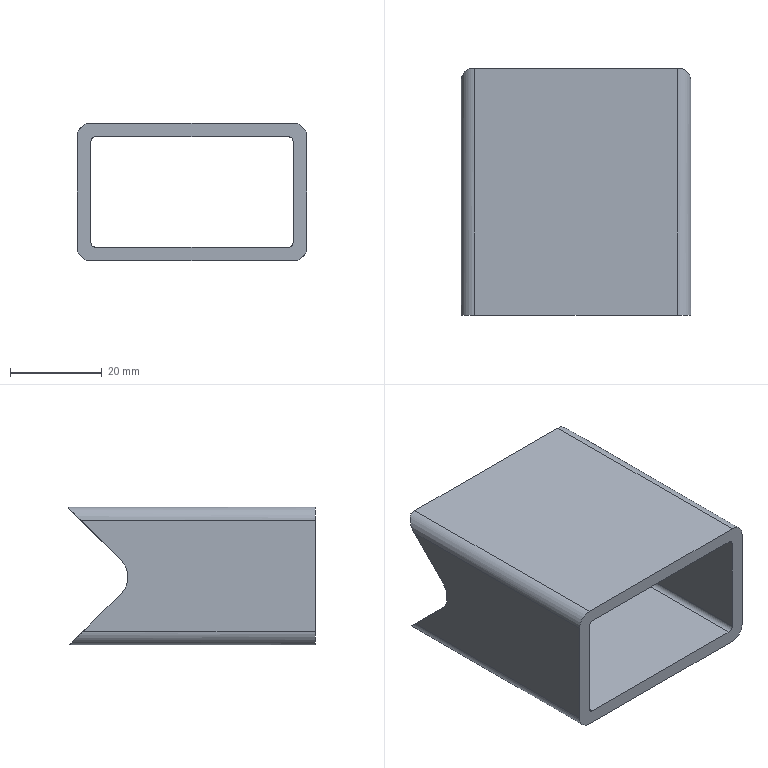Part | SolidWorks | features Fillet 2, Extrusion 1, ICE 1, Shell 1 | 1 solid | 22 faces | box 50 x 53.7 x 30 mm | volume 21768 mm3 | plane 12 | cylinder 10 | commonest cylinder face diameters 2 x4 6 x4 10 x2
STEP:
#1=CARTESIAN_POINT('',(23.24,26.85,29.732));
#2=VERTEX_POINT('',#1);
#3=CARTESIAN_POINT('',(-23.24,26.85,29.732));
#4=VERTEX_POINT('',#3);
#5=CARTESIAN_POINT('',(-25.,26.85,29.732));
#6=DIRECTION('',(-1.,0.,0.));
#7=VECTOR('',#6,1000.);
#8=LINE('',#5,#7);
#9=EDGE_CURVE('',#2,#4,#8,.T.);
#10=ORIENTED_EDGE('',*,*,#9,.T.);
#11=CARTESIAN_POINT('',(-22.,26.85,30.));
#12=VERTEX_POINT('',#11);
#13=CARTESIAN_POINT('',(-22.,26.85,27.));
#14=DIRECTION('',(0.,1.,0.));
#15=DIRECTION('',(0.,0.,-1.));
#16=AXIS2_PLACEMENT_3D('',#13,#14,#15);
#17=CIRCLE('',#16,3.);
#18=EDGE_CURVE('',#4,#12,#17,.T.);
#19=ORIENTED_EDGE('',*,*,#18,.T.);
#20=CARTESIAN_POINT('',(22.,26.85,30.));
#21=VERTEX_POINT('',#20);
#22=CARTESIAN_POINT('',(-25.,26.85,30.));
#23=DIRECTION('',(-1.,0.,0.));
#24=VECTOR('',#23,1000.);
#25=LINE('',#22,#24);
#26=EDGE_CURVE('',#21,#12,#25,.T.);
#27=ORIENTED_EDGE('',*,*,#26,.F.);
#28=CARTESIAN_POINT('',(22.,26.85,27.));
#29=DIRECTION('',(0.,1.,0.));
#30=DIRECTION('',(0.,0.,-1.));
#31=AXIS2_PLACEMENT_3D('',#28,#29,#30);
#32=CIRCLE('',#31,3.);
#33=EDGE_CURVE('',#21,#2,#32,.T.);
#34=ORIENTED_EDGE('',*,*,#33,.T.);
#35=EDGE_LOOP('',(#10,#19,#27,#34));
#36=FACE_OUTER_BOUND('',#35,.T.);
#37=CARTESIAN_POINT('',(-25.,26.85,30.));
#38=DIRECTION('',(0.,-1.,0.));
#39=DIRECTION('',(0.,0.,-1.));
#40=AXIS2_PLACEMENT_3D('',#37,#38,#39);
#41=PLANE('',#40);
#42=ADVANCED_FACE('',(#36),#41,.F.);
#43=CARTESIAN_POINT('',(-25.,-26.85,27.));
#44=VERTEX_POINT('',#43);
#45=CARTESIAN_POINT('',(-25.,-26.85,3.));
#46=VERTEX_POINT('',#45);
#47=CARTESIAN_POINT('',(-25.,-26.85,30.));
#48=DIRECTION('',(0.,0.,-1.));
#49=VECTOR('',#48,1000.);
#50=LINE('',#47,#49);
#51=EDGE_CURVE('',#44,#46,#50,.T.);
#52=ORIENTED_EDGE('',*,*,#51,.T.);
#53=CARTESIAN_POINT('',(-22.,-26.85,0.));
#54=VERTEX_POINT('',#53);
#55=CARTESIAN_POINT('',(-22.,-26.85,3.));
#56=DIRECTION('',(0.,-1.,0.));
#57=DIRECTION('',(0.,0.,1.));
#58=AXIS2_PLACEMENT_3D('',#55,#56,#57);
#59=CIRCLE('',#58,3.);
#60=EDGE_CURVE('',#46,#54,#59,.T.);
#61=ORIENTED_EDGE('',*,*,#60,.T.);
#62=CARTESIAN_POINT('',(22.,-26.85,0.));
#63=VERTEX_POINT('',#62);
#64=CARTESIAN_POINT('',(-25.,-26.85,0.));
#65=DIRECTION('',(1.,0.,0.));
#66=VECTOR('',#65,1000.);
#67=LINE('',#64,#66);
#68=EDGE_CURVE('',#54,#63,#67,.T.);
#69=ORIENTED_EDGE('',*,*,#68,.T.);
#70=CARTESIAN_POINT('',(25.,-26.85,3.));
#71=VERTEX_POINT('',#70);
#72=CARTESIAN_POINT('',(22.,-26.85,3.));
#73=DIRECTION('',(0.,-1.,0.));
#74=DIRECTION('',(0.,0.,1.));
#75=AXIS2_PLACEMENT_3D('',#72,#73,#74);
#76=CIRCLE('',#75,3.);
#77=EDGE_CURVE('',#63,#71,#76,.T.);
#78=ORIENTED_EDGE('',*,*,#77,.T.);
#79=CARTESIAN_POINT('',(25.,-26.85,27.));
#80=VERTEX_POINT('',#79);
#81=CARTESIAN_POINT('',(25.,-26.85,30.));
#82=DIRECTION('',(0.,0.,-1.));
#83=VECTOR('',#82,1000.);
#84=LINE('',#81,#83);
#85=EDGE_CURVE('',#80,#71,#84,.T.);
#86=ORIENTED_EDGE('',*,*,#85,.F.);
#87=CARTESIAN_POINT('',(22.,-26.85,30.));
#88=VERTEX_POINT('',#87);
#89=CARTESIAN_POINT('',(22.,-26.85,27.));
#90=DIRECTION('',(0.,-1.,0.));
#91=DIRECTION('',(0.,0.,1.));
#92=AXIS2_PLACEMENT_3D('',#89,#90,#91);
#93=CIRCLE('',#92,3.);
#94=EDGE_CURVE('',#80,#88,#93,.T.);
#95=ORIENTED_EDGE('',*,*,#94,.T.);
#96=CARTESIAN_POINT('',(-22.,-26.85,30.));
#97=VERTEX_POINT('',#96);
#98=CARTESIAN_POINT('',(-25.,-26.85,30.));
#99=DIRECTION('',(1.,0.,0.));
#100=VECTOR('',#99,1000.);
#101=LINE('',#98,#100);
#102=EDGE_CURVE('',#97,#88,#101,.T.);
#103=ORIENTED_EDGE('',*,*,#102,.F.);
#104=CARTESIAN_POINT('',(-22.,-26.85,27.));
#105=DIRECTION('',(0.,-1.,0.));
#106=DIRECTION('',(0.,0.,1.));
#107=AXIS2_PLACEMENT_3D('',#104,#105,#106);
#108=CIRCLE('',#107,3.);
#109=EDGE_CURVE('',#97,#44,#108,.T.);
#110=ORIENTED_EDGE('',*,*,#109,.T.);
#111=EDGE_LOOP('',(#52,#61,#69,#78,#86,#95,#103,#110));
#112=FACE_OUTER_BOUND('',#111,.T.);
#113=CARTESIAN_POINT('',(-21.,-26.85,3.));
#114=VERTEX_POINT('',#113);
#115=CARTESIAN_POINT('',(21.,-26.85,3.));
#116=VERTEX_POINT('',#115);
#117=CARTESIAN_POINT('',(-25.,-26.85,3.));
#118=DIRECTION('',(1.,0.,0.));
#119=VECTOR('',#118,1000.);
#120=LINE('',#117,#119);
#121=EDGE_CURVE('',#114,#116,#120,.T.);
#122=ORIENTED_EDGE('',*,*,#121,.F.);
#123=CARTESIAN_POINT('',(-22.,-26.85,4.));
#124=VERTEX_POINT('',#123);
#125=CARTESIAN_POINT('',(-21.,-26.85,4.));
#126=DIRECTION('',(0.,1.,0.));
#127=DIRECTION('',(0.,0.,1.));
#128=AXIS2_PLACEMENT_3D('',#125,#126,#127);
#129=CIRCLE('',#128,1.);
#130=EDGE_CURVE('',#114,#124,#129,.T.);
#131=ORIENTED_EDGE('',*,*,#130,.T.);
#132=CARTESIAN_POINT('',(-22.,-26.85,26.));
#133=VERTEX_POINT('',#132);
#134=CARTESIAN_POINT('',(-22.,-26.85,30.));
#135=DIRECTION('',(0.,0.,-1.));
#136=VECTOR('',#135,1000.);
#137=LINE('',#134,#136);
#138=EDGE_CURVE('',#133,#124,#137,.T.);
#139=ORIENTED_EDGE('',*,*,#138,.F.);
#140=CARTESIAN_POINT('',(-21.,-26.85,27.));
#141=VERTEX_POINT('',#140);
#142=CARTESIAN_POINT('',(-21.,-26.85,26.));
#143=DIRECTION('',(0.,1.,0.));
#144=DIRECTION('',(0.,0.,1.));
#145=AXIS2_PLACEMENT_3D('',#142,#143,#144);
#146=CIRCLE('',#145,1.);
#147=EDGE_CURVE('',#133,#141,#146,.T.);
#148=ORIENTED_EDGE('',*,*,#147,.T.);
#149=CARTESIAN_POINT('',(21.,-26.85,27.));
#150=VERTEX_POINT('',#149);
#151=CARTESIAN_POINT('',(-25.,-26.85,27.));
#152=DIRECTION('',(1.,0.,0.));
#153=VECTOR('',#152,1000.);
#154=LINE('',#151,#153);
#155=EDGE_CURVE('',#141,#150,#154,.T.);
#156=ORIENTED_EDGE('',*,*,#155,.T.);
#157=CARTESIAN_POINT('',(22.,-26.85,26.));
#158=VERTEX_POINT('',#157);
#159=CARTESIAN_POINT('',(21.,-26.85,26.));
#160=DIRECTION('',(0.,1.,0.));
#161=DIRECTION('',(0.,0.,1.));
#162=AXIS2_PLACEMENT_3D('',#159,#160,#161);
#163=CIRCLE('',#162,1.);
#164=EDGE_CURVE('',#150,#158,#163,.T.);
#165=ORIENTED_EDGE('',*,*,#164,.T.);
#166=CARTESIAN_POINT('',(22.,-26.85,4.));
#167=VERTEX_POINT('',#166);
#168=CARTESIAN_POINT('',(22.,-26.85,30.));
#169=DIRECTION('',(0.,0.,-1.));
#170=VECTOR('',#169,1000.);
#171=LINE('',#168,#170);
#172=EDGE_CURVE('',#158,#167,#171,.T.);
#173=ORIENTED_EDGE('',*,*,#172,.T.);
#174=CARTESIAN_POINT('',(21.,-26.85,4.));
#175=DIRECTION('',(0.,1.,0.));
#176=DIRECTION('',(0.,0.,1.));
#177=AXIS2_PLACEMENT_3D('',#174,#175,#176);
#178=CIRCLE('',#177,1.);
#179=EDGE_CURVE('',#167,#116,#178,.T.);
#180=ORIENTED_EDGE('',*,*,#179,.T.);
#181=EDGE_LOOP('',(#122,#131,#139,#148,#156,#165,#173,#180));
#182=FACE_BOUND('',#181,.T.);
#183=CARTESIAN_POINT('',(-25.,-26.85,30.));
#184=DIRECTION('',(0.,1.,0.));
#185=DIRECTION('',(0.,0.,1.));
#186=AXIS2_PLACEMENT_3D('',#183,#184,#185);
#187=PLANE('',#186);
#188=ADVANCED_FACE('',(#112,#182),#187,.F.);
#189=ORIENTED_EDGE('',*,*,#85,.T.);
#190=CARTESIAN_POINT('',(25.,23.613,3.));
#191=VERTEX_POINT('',#190);
#192=CARTESIAN_POINT('',(25.,26.85,3.));
#193=DIRECTION('',(0.,1.,0.));
#194=VECTOR('',#193,1000.);
#195=LINE('',#192,#194);
#196=EDGE_CURVE('',#71,#191,#195,.T.);
#197=ORIENTED_EDGE('',*,*,#196,.T.);
#198=CARTESIAN_POINT('',(25.,15.401,11.212));
#199=VERTEX_POINT('',#198);
#200=CARTESIAN_POINT('',(25.,15.401,11.212));
#201=DIRECTION('',(0.,0.7071,-0.7071));
#202=VECTOR('',#201,1000.);
#203=LINE('',#200,#202);
#204=EDGE_CURVE('',#199,#191,#203,.T.);
#205=ORIENTED_EDGE('',*,*,#204,.F.);
#206=CARTESIAN_POINT('',(25.,15.401,18.283));
#207=VERTEX_POINT('',#206);
#208=CARTESIAN_POINT('',(25.,18.937,14.748));
#209=DIRECTION('',(1.,0.,0.));
#210=DIRECTION('',(0.,1.,0.));
#211=AXIS2_PLACEMENT_3D('',#208,#209,#210);
#212=CIRCLE('',#211,5.);
#213=EDGE_CURVE('',#207,#199,#212,.T.);
#214=ORIENTED_EDGE('',*,*,#213,.F.);
#215=CARTESIAN_POINT('',(25.,24.118,27.));
#216=VERTEX_POINT('',#215);
#217=CARTESIAN_POINT('',(25.,15.401,18.283));
#218=DIRECTION('',(0.,-0.7071,-0.7071));
#219=VECTOR('',#218,1000.);
#220=LINE('',#217,#219);
#221=EDGE_CURVE('',#216,#207,#220,.T.);
#222=ORIENTED_EDGE('',*,*,#221,.F.);
#223=CARTESIAN_POINT('',(25.,-26.85,27.));
#224=DIRECTION('',(0.,-1.,0.));
#225=VECTOR('',#224,1000.);
#226=LINE('',#223,#225);
#227=EDGE_CURVE('',#216,#80,#226,.T.);
#228=ORIENTED_EDGE('',*,*,#227,.T.);
#229=EDGE_LOOP('',(#189,#197,#205,#214,#222,#228));
#230=FACE_OUTER_BOUND('',#229,.T.);
#231=CARTESIAN_POINT('',(25.,26.85,30.));
#232=DIRECTION('',(-1.,0.,0.));
#233=DIRECTION('',(0.,-1.,0.));
#234=AXIS2_PLACEMENT_3D('',#231,#232,#233);
#235=PLANE('',#234);
#236=ADVANCED_FACE('',(#230),#235,.F.);
#237=CARTESIAN_POINT('',(-25.,15.401,11.212));
#238=VERTEX_POINT('',#237);
#239=CARTESIAN_POINT('',(-25.,23.613,3.));
#240=VERTEX_POINT('',#239);
#241=CARTESIAN_POINT('',(-25.,11.732,14.882));
#242=DIRECTION('',(0.,0.7071,-0.7071));
#243=VECTOR('',#242,1000.);
#244=LINE('',#241,#243);
#245=EDGE_CURVE('',#238,#240,#244,.T.);
#246=ORIENTED_EDGE('',*,*,#245,.T.);
#247=CARTESIAN_POINT('',(-25.,26.85,3.));
#248=DIRECTION('',(0.,-1.,0.));
#249=VECTOR('',#248,1000.);
#250=LINE('',#247,#249);
#251=EDGE_CURVE('',#240,#46,#250,.T.);
#252=ORIENTED_EDGE('',*,*,#251,.T.);
#253=ORIENTED_EDGE('',*,*,#51,.F.);
#254=CARTESIAN_POINT('',(-25.,24.118,27.));
#255=VERTEX_POINT('',#254);
#256=CARTESIAN_POINT('',(-25.,26.85,27.));
#257=DIRECTION('',(0.,1.,0.));
#258=VECTOR('',#257,1000.);
#259=LINE('',#256,#258);
#260=EDGE_CURVE('',#44,#255,#259,.T.);
#261=ORIENTED_EDGE('',*,*,#260,.T.);
#262=CARTESIAN_POINT('',(-25.,15.401,18.283));
#263=VERTEX_POINT('',#262);
#264=CARTESIAN_POINT('',(-25.,26.984,29.866));
#265=DIRECTION('',(0.,-0.7071,-0.7071));
#266=VECTOR('',#265,1000.);
#267=LINE('',#264,#266);
#268=EDGE_CURVE('',#255,#263,#267,.T.);
#269=ORIENTED_EDGE('',*,*,#268,.T.);
#270=CARTESIAN_POINT('',(-25.,18.937,14.748));
#271=DIRECTION('',(1.,0.,0.));
#272=DIRECTION('',(0.,1.,0.));
#273=AXIS2_PLACEMENT_3D('',#270,#271,#272);
#274=CIRCLE('',#273,5.);
#275=EDGE_CURVE('',#263,#238,#274,.T.);
#276=ORIENTED_EDGE('',*,*,#275,.T.);
#277=EDGE_LOOP('',(#246,#252,#253,#261,#269,#276));
#278=FACE_OUTER_BOUND('',#277,.T.);
#279=CARTESIAN_POINT('',(-25.,26.85,30.));
#280=DIRECTION('',(1.,0.,0.));
#281=DIRECTION('',(0.,1.,0.));
#282=AXIS2_PLACEMENT_3D('',#279,#280,#281);
#283=PLANE('',#282);
#284=ADVANCED_FACE('',(#278),#283,.F.);
#285=ORIENTED_EDGE('',*,*,#26,.T.);
#286=CARTESIAN_POINT('',(-22.,-26.85,30.));
#287=DIRECTION('',(0.,-1.,0.));
#288=VECTOR('',#287,1000.);
#289=LINE('',#286,#288);
#290=EDGE_CURVE('',#12,#97,#289,.T.);
#291=ORIENTED_EDGE('',*,*,#290,.T.);
#292=ORIENTED_EDGE('',*,*,#102,.T.);
#293=CARTESIAN_POINT('',(22.,26.85,30.));
#294=DIRECTION('',(0.,1.,0.));
#295=VECTOR('',#294,1000.);
#296=LINE('',#293,#295);
#297=EDGE_CURVE('',#88,#21,#296,.T.);
#298=ORIENTED_EDGE('',*,*,#297,.T.);
#299=EDGE_LOOP('',(#285,#291,#292,#298));
#300=FACE_OUTER_BOUND('',#299,.T.);
#301=CARTESIAN_POINT('',(0.,0.,30.));
#302=DIRECTION('',(0.,0.,1.));
#303=DIRECTION('',(1.,0.,0.));
#304=AXIS2_PLACEMENT_3D('',#301,#302,#303);
#305=PLANE('',#304);
#306=ADVANCED_FACE('',(#300),#305,.T.);
#307=ORIENTED_EDGE('',*,*,#68,.F.);
#308=CARTESIAN_POINT('',(-22.,26.613,0.));
#309=VERTEX_POINT('',#308);
#310=CARTESIAN_POINT('',(-22.,0.,0.));
#311=DIRECTION('',(0.,1.,0.));
#312=VECTOR('',#311,1000.);
#313=LINE('',#310,#312);
#314=EDGE_CURVE('',#54,#309,#313,.T.);
#315=ORIENTED_EDGE('',*,*,#314,.T.);
#316=CARTESIAN_POINT('',(22.,26.613,0.));
#317=VERTEX_POINT('',#316);
#318=CARTESIAN_POINT('',(0.,26.613,0.));
#319=DIRECTION('',(1.,0.,0.));
#320=VECTOR('',#319,1000.);
#321=LINE('',#318,#320);
#322=EDGE_CURVE('',#309,#317,#321,.T.);
#323=ORIENTED_EDGE('',*,*,#322,.T.);
#324=CARTESIAN_POINT('',(22.,0.,0.));
#325=DIRECTION('',(0.,-1.,0.));
#326=VECTOR('',#325,1000.);
#327=LINE('',#324,#326);
#328=EDGE_CURVE('',#317,#63,#327,.T.);
#329=ORIENTED_EDGE('',*,*,#328,.T.);
#330=EDGE_LOOP('',(#307,#315,#323,#329));
#331=FACE_OUTER_BOUND('',#330,.T.);
#332=CARTESIAN_POINT('',(0.,0.,0.));
#333=DIRECTION('',(0.,0.,1.));
#334=DIRECTION('',(1.,0.,0.));
#335=AXIS2_PLACEMENT_3D('',#332,#333,#334);
#336=PLANE('',#335);
#337=ADVANCED_FACE('',(#331),#336,.F.);
#338=CARTESIAN_POINT('',(22.,22.613,4.));
#339=VERTEX_POINT('',#338);
#340=CARTESIAN_POINT('',(22.,15.401,11.212));
#341=VERTEX_POINT('',#340);
#342=CARTESIAN_POINT('',(22.,11.732,14.882));
#343=DIRECTION('',(0.,-0.7071,0.7071));
#344=VECTOR('',#343,1000.);
#345=LINE('',#342,#344);
#346=EDGE_CURVE('',#339,#341,#345,.T.);
#347=ORIENTED_EDGE('',*,*,#346,.F.);
#348=CARTESIAN_POINT('',(22.,-26.85,4.));
#349=DIRECTION('',(0.,-1.,0.));
#350=VECTOR('',#349,1000.);
#351=LINE('',#348,#350);
#352=EDGE_CURVE('',#339,#167,#351,.T.);
#353=ORIENTED_EDGE('',*,*,#352,.T.);
#354=ORIENTED_EDGE('',*,*,#172,.F.);
#355=CARTESIAN_POINT('',(22.,23.118,26.));
#356=VERTEX_POINT('',#355);
#357=CARTESIAN_POINT('',(22.,26.85,26.));
#358=DIRECTION('',(0.,1.,0.));
#359=VECTOR('',#358,1000.);
#360=LINE('',#357,#359);
#361=EDGE_CURVE('',#158,#356,#360,.T.);
#362=ORIENTED_EDGE('',*,*,#361,.T.);
#363=CARTESIAN_POINT('',(22.,15.401,18.283));
#364=VERTEX_POINT('',#363);
#365=CARTESIAN_POINT('',(22.,26.984,29.866));
#366=DIRECTION('',(0.,0.7071,0.7071));
#367=VECTOR('',#366,1000.);
#368=LINE('',#365,#367);
#369=EDGE_CURVE('',#364,#356,#368,.T.);
#370=ORIENTED_EDGE('',*,*,#369,.F.);
#371=CARTESIAN_POINT('',(22.,18.937,14.748));
#372=DIRECTION('',(-1.,0.,0.));
#373=DIRECTION('',(0.,-1.,0.));
#374=AXIS2_PLACEMENT_3D('',#371,#372,#373);
#375=CIRCLE('',#374,5.);
#376=EDGE_CURVE('',#341,#364,#375,.T.);
#377=ORIENTED_EDGE('',*,*,#376,.F.);
#378=EDGE_LOOP('',(#347,#353,#354,#362,#370,#377));
#379=FACE_OUTER_BOUND('',#378,.T.);
#380=CARTESIAN_POINT('',(22.,26.85,30.));
#381=DIRECTION('',(-1.,0.,0.));
#382=DIRECTION('',(0.,-1.,0.));
#383=AXIS2_PLACEMENT_3D('',#380,#381,#382);
#384=PLANE('',#383);
#385=ADVANCED_FACE('',(#379),#384,.T.);
#386=ORIENTED_EDGE('',*,*,#138,.T.);
#387=CARTESIAN_POINT('',(-22.,22.613,4.));
#388=VERTEX_POINT('',#387);
#389=CARTESIAN_POINT('',(-22.,23.613,4.));
#390=DIRECTION('',(0.,1.,0.));
#391=VECTOR('',#390,1000.);
#392=LINE('',#389,#391);
#393=EDGE_CURVE('',#124,#388,#392,.T.);
#394=ORIENTED_EDGE('',*,*,#393,.T.);
#395=CARTESIAN_POINT('',(-22.,15.401,11.212));
#396=VERTEX_POINT('',#395);
#397=CARTESIAN_POINT('',(-22.,11.732,14.882));
#398=DIRECTION('',(0.,0.7071,-0.7071));
#399=VECTOR('',#398,1000.);
#400=LINE('',#397,#399);
#401=EDGE_CURVE('',#396,#388,#400,.T.);
#402=ORIENTED_EDGE('',*,*,#401,.F.);
#403=CARTESIAN_POINT('',(-22.,15.401,18.283));
#404=VERTEX_POINT('',#403);
#405=CARTESIAN_POINT('',(-22.,18.937,14.748));
#406=DIRECTION('',(1.,0.,0.));
#407=DIRECTION('',(0.,1.,0.));
#408=AXIS2_PLACEMENT_3D('',#405,#406,#407);
#409=CIRCLE('',#408,5.);
#410=EDGE_CURVE('',#404,#396,#409,.T.);
#411=ORIENTED_EDGE('',*,*,#410,.F.);
#412=CARTESIAN_POINT('',(-22.,23.118,26.));
#413=VERTEX_POINT('',#412);
#414=CARTESIAN_POINT('',(-22.,26.984,29.866));
#415=DIRECTION('',(0.,-0.7071,-0.7071));
#416=VECTOR('',#415,1000.);
#417=LINE('',#414,#416);
#418=EDGE_CURVE('',#413,#404,#417,.T.);
#419=ORIENTED_EDGE('',*,*,#418,.F.);
#420=CARTESIAN_POINT('',(-22.,26.85,26.));
#421=DIRECTION('',(0.,-1.,0.));
#422=VECTOR('',#421,1000.);
#423=LINE('',#420,#422);
#424=EDGE_CURVE('',#413,#133,#423,.T.);
#425=ORIENTED_EDGE('',*,*,#424,.T.);
#426=EDGE_LOOP('',(#386,#394,#402,#411,#419,#425));
#427=FACE_OUTER_BOUND('',#426,.T.);
#428=CARTESIAN_POINT('',(-22.,26.85,30.));
#429=DIRECTION('',(1.,0.,0.));
#430=DIRECTION('',(0.,1.,0.));
#431=AXIS2_PLACEMENT_3D('',#428,#429,#430);
#432=PLANE('',#431);
#433=ADVANCED_FACE('',(#427),#432,.T.);
#434=ORIENTED_EDGE('',*,*,#155,.F.);
#435=CARTESIAN_POINT('',(-21.,24.118,27.));
#436=VERTEX_POINT('',#435);
#437=CARTESIAN_POINT('',(-21.,0.,27.));
#438=DIRECTION('',(0.,1.,0.));
#439=VECTOR('',#438,1000.);
#440=LINE('',#437,#439);
#441=EDGE_CURVE('',#141,#436,#440,.T.);
#442=ORIENTED_EDGE('',*,*,#441,.T.);
#443=CARTESIAN_POINT('',(21.,24.118,27.));
#444=VERTEX_POINT('',#443);
#445=CARTESIAN_POINT('',(0.,24.118,27.));
#446=DIRECTION('',(1.,0.,0.));
#447=VECTOR('',#446,1000.);
#448=LINE('',#445,#447);
#449=EDGE_CURVE('',#436,#444,#448,.T.);
#450=ORIENTED_EDGE('',*,*,#449,.T.);
#451=CARTESIAN_POINT('',(21.,0.,27.));
#452=DIRECTION('',(0.,-1.,0.));
#453=VECTOR('',#452,1000.);
#454=LINE('',#451,#453);
#455=EDGE_CURVE('',#444,#150,#454,.T.);
#456=ORIENTED_EDGE('',*,*,#455,.T.);
#457=EDGE_LOOP('',(#434,#442,#450,#456));
#458=FACE_OUTER_BOUND('',#457,.T.);
#459=CARTESIAN_POINT('',(0.,0.,27.));
#460=DIRECTION('',(0.,0.,1.));
#461=DIRECTION('',(1.,0.,0.));
#462=AXIS2_PLACEMENT_3D('',#459,#460,#461);
#463=PLANE('',#462);
#464=ADVANCED_FACE('',(#458),#463,.F.);
#465=CARTESIAN_POINT('',(-21.,23.613,3.));
#466=VERTEX_POINT('',#465);
#467=CARTESIAN_POINT('',(21.,23.613,3.));
#468=VERTEX_POINT('',#467);
#469=CARTESIAN_POINT('',(0.,23.613,3.));
#470=DIRECTION('',(1.,0.,0.));
#471=VECTOR('',#470,1000.);
#472=LINE('',#469,#471);
#473=EDGE_CURVE('',#466,#468,#472,.T.);
#474=ORIENTED_EDGE('',*,*,#473,.F.);
#475=CARTESIAN_POINT('',(-21.,-26.85,3.));
#476=DIRECTION('',(0.,-1.,0.));
#477=VECTOR('',#476,1000.);
#478=LINE('',#475,#477);
#479=EDGE_CURVE('',#466,#114,#478,.T.);
#480=ORIENTED_EDGE('',*,*,#479,.T.);
#481=ORIENTED_EDGE('',*,*,#121,.T.);
#482=CARTESIAN_POINT('',(21.,23.613,3.));
#483=DIRECTION('',(0.,1.,0.));
#484=VECTOR('',#483,1000.);
#485=LINE('',#482,#484);
#486=EDGE_CURVE('',#116,#468,#485,.T.);
#487=ORIENTED_EDGE('',*,*,#486,.T.);
#488=EDGE_LOOP('',(#474,#480,#481,#487));
#489=FACE_OUTER_BOUND('',#488,.T.);
#490=CARTESIAN_POINT('',(0.,0.,3.));
#491=DIRECTION('',(0.,0.,1.));
#492=DIRECTION('',(1.,0.,0.));
#493=AXIS2_PLACEMENT_3D('',#490,#491,#492);
#494=PLANE('',#493);
#495=ADVANCED_FACE('',(#489),#494,.T.);
#496=CARTESIAN_POINT('',(-41.,15.401,18.283));
#497=DIRECTION('',(1.,0.,0.));
#498=VECTOR('',#497,1000.);
#499=LINE('',#496,#498);
#500=EDGE_CURVE('',#263,#404,#499,.T.);
#501=ORIENTED_EDGE('',*,*,#500,.T.);
#502=ORIENTED_EDGE('',*,*,#410,.T.);
#503=CARTESIAN_POINT('',(-41.,15.401,11.212));
#504=DIRECTION('',(1.,0.,0.));
#505=VECTOR('',#504,1000.);
#506=LINE('',#503,#505);
#507=EDGE_CURVE('',#238,#396,#506,.T.);
#508=ORIENTED_EDGE('',*,*,#507,.F.);
#509=ORIENTED_EDGE('',*,*,#275,.F.);
#510=EDGE_LOOP('',(#501,#502,#508,#509));
#511=FACE_OUTER_BOUND('',#510,.T.);
#512=CARTESIAN_POINT('',(-41.,18.937,14.748));
#513=DIRECTION('',(1.,0.,0.));
#514=DIRECTION('',(0.,1.,0.));
#515=AXIS2_PLACEMENT_3D('',#512,#513,#514);
#516=CYLINDRICAL_SURFACE('',#515,5.);
#517=ADVANCED_FACE('',(#511),#516,.F.);
#518=ORIENTED_EDGE('',*,*,#376,.T.);
#519=CARTESIAN_POINT('',(-41.,15.401,18.283));
#520=DIRECTION('',(1.,0.,0.));
#521=VECTOR('',#520,1000.);
#522=LINE('',#519,#521);
#523=EDGE_CURVE('',#364,#207,#522,.T.);
#524=ORIENTED_EDGE('',*,*,#523,.T.);
#525=ORIENTED_EDGE('',*,*,#213,.T.);
#526=CARTESIAN_POINT('',(-41.,15.401,11.212));
#527=DIRECTION('',(1.,0.,0.));
#528=VECTOR('',#527,1000.);
#529=LINE('',#526,#528);
#530=EDGE_CURVE('',#341,#199,#529,.T.);
#531=ORIENTED_EDGE('',*,*,#530,.F.);
#532=EDGE_LOOP('',(#518,#524,#525,#531));
#533=FACE_OUTER_BOUND('',#532,.T.);
#534=CARTESIAN_POINT('',(-41.,18.937,14.748));
#535=DIRECTION('',(1.,0.,0.));
#536=DIRECTION('',(0.,1.,0.));
#537=AXIS2_PLACEMENT_3D('',#534,#535,#536);
#538=CYLINDRICAL_SURFACE('',#537,5.);
#539=ADVANCED_FACE('',(#533),#538,.F.);
#540=ORIENTED_EDGE('',*,*,#268,.F.);
#541=CARTESIAN_POINT('',(-25.,24.118,27.));
#542=CARTESIAN_POINT('',(-25.,25.33,28.212));
#543=CARTESIAN_POINT('',(-24.343,26.349,29.231));
#544=CARTESIAN_POINT('',(-23.24,26.85,29.732));
#545=(BOUNDED_CURVE()B_SPLINE_CURVE(3,(#541,#542,#543,#544),.UNSPECIFIED.,.F.,.T.)B_SPLINE_CURVE_WITH_KNOTS((4,4),(4.712,5.857),.UNSPECIFIED.)CURVE()GEOMETRIC_REPRESENTATION_ITEM()RATIONAL_B_SPLINE_CURVE((1.,0.8937,0.8937,1.))REPRESENTATION_ITEM(''));
#546=EDGE_CURVE('',#255,#4,#545,.T.);
#547=ORIENTED_EDGE('',*,*,#546,.T.);
#548=ORIENTED_EDGE('',*,*,#9,.F.);
#549=CARTESIAN_POINT('',(23.24,26.85,29.732));
#550=CARTESIAN_POINT('',(24.343,26.349,29.231));
#551=CARTESIAN_POINT('',(25.,25.33,28.212));
#552=CARTESIAN_POINT('',(25.,24.118,27.));
#553=(BOUNDED_CURVE()B_SPLINE_CURVE(3,(#549,#550,#551,#552),.UNSPECIFIED.,.F.,.F.)B_SPLINE_CURVE_WITH_KNOTS((4,4),(3.568,4.712),.UNSPECIFIED.)CURVE()GEOMETRIC_REPRESENTATION_ITEM()RATIONAL_B_SPLINE_CURVE((1.,0.8937,0.8937,1.))REPRESENTATION_ITEM(''));
#554=EDGE_CURVE('',#2,#216,#553,.T.);
#555=ORIENTED_EDGE('',*,*,#554,.T.);
#556=ORIENTED_EDGE('',*,*,#221,.T.);
#557=ORIENTED_EDGE('',*,*,#523,.F.);
#558=ORIENTED_EDGE('',*,*,#369,.T.);
#559=CARTESIAN_POINT('',(22.,23.118,26.));
#560=CARTESIAN_POINT('',(22.,23.704,26.586));
#561=CARTESIAN_POINT('',(21.586,24.118,27.));
#562=CARTESIAN_POINT('',(21.,24.118,27.));
#563=(BOUNDED_CURVE()B_SPLINE_CURVE(3,(#559,#560,#561,#562),.UNSPECIFIED.,.F.,.F.)B_SPLINE_CURVE_WITH_KNOTS((4,4),(4.712,6.283),.UNSPECIFIED.)CURVE()GEOMETRIC_REPRESENTATION_ITEM()RATIONAL_B_SPLINE_CURVE((1.,0.8047,0.8047,1.))REPRESENTATION_ITEM(''));
#564=EDGE_CURVE('',#356,#444,#563,.T.);
#565=ORIENTED_EDGE('',*,*,#564,.T.);
#566=ORIENTED_EDGE('',*,*,#449,.F.);
#567=CARTESIAN_POINT('',(-21.,24.118,27.));
#568=CARTESIAN_POINT('',(-21.586,24.118,27.));
#569=CARTESIAN_POINT('',(-22.,23.704,26.586));
#570=CARTESIAN_POINT('',(-22.,23.118,26.));
#571=(BOUNDED_CURVE()B_SPLINE_CURVE(3,(#567,#568,#569,#570),.UNSPECIFIED.,.F.,.F.)B_SPLINE_CURVE_WITH_KNOTS((4,4),(3.142,4.712),.UNSPECIFIED.)CURVE()GEOMETRIC_REPRESENTATION_ITEM()RATIONAL_B_SPLINE_CURVE((1.,0.8047,0.8047,1.))REPRESENTATION_ITEM(''));
#572=EDGE_CURVE('',#436,#413,#571,.T.);
#573=ORIENTED_EDGE('',*,*,#572,.T.);
#574=ORIENTED_EDGE('',*,*,#418,.T.);
#575=ORIENTED_EDGE('',*,*,#500,.F.);
#576=EDGE_LOOP('',(#540,#547,#548,#555,#556,#557,#558,#565,#566,#573,#574,#575));
#577=FACE_OUTER_BOUND('',#576,.T.);
#578=CARTESIAN_POINT('',(-41.,15.401,18.283));
#579=DIRECTION('',(0.,-0.7071,0.7071));
#580=DIRECTION('',(0.,-0.7071,-0.7071));
#581=AXIS2_PLACEMENT_3D('',#578,#579,#580);
#582=PLANE('',#581);
#583=ADVANCED_FACE('',(#577),#582,.F.);
#584=ORIENTED_EDGE('',*,*,#322,.F.);
#585=CARTESIAN_POINT('',(-22.,26.613,0.));
#586=CARTESIAN_POINT('',(-23.757,26.613,0.));
#587=CARTESIAN_POINT('',(-25.,25.371,1.243));
#588=CARTESIAN_POINT('',(-25.,23.613,3.));
#589=(BOUNDED_CURVE()B_SPLINE_CURVE(3,(#585,#586,#587,#588),.UNSPECIFIED.,.F.,.F.)B_SPLINE_CURVE_WITH_KNOTS((4,4),(3.142,4.712),.UNSPECIFIED.)CURVE()GEOMETRIC_REPRESENTATION_ITEM()RATIONAL_B_SPLINE_CURVE((1.,0.8047,0.8047,1.))REPRESENTATION_ITEM(''));
#590=EDGE_CURVE('',#309,#240,#589,.T.);
#591=ORIENTED_EDGE('',*,*,#590,.T.);
#592=ORIENTED_EDGE('',*,*,#245,.F.);
#593=ORIENTED_EDGE('',*,*,#507,.T.);
#594=ORIENTED_EDGE('',*,*,#401,.T.);
#595=CARTESIAN_POINT('',(-22.,22.613,4.));
#596=CARTESIAN_POINT('',(-22.,23.199,3.414));
#597=CARTESIAN_POINT('',(-21.586,23.613,3.));
#598=CARTESIAN_POINT('',(-21.,23.613,3.));
#599=(BOUNDED_CURVE()B_SPLINE_CURVE(3,(#595,#596,#597,#598),.UNSPECIFIED.,.F.,.F.)B_SPLINE_CURVE_WITH_KNOTS((4,4),(4.712,6.283),.UNSPECIFIED.)CURVE()GEOMETRIC_REPRESENTATION_ITEM()RATIONAL_B_SPLINE_CURVE((1.,0.8047,0.8047,1.))REPRESENTATION_ITEM(''));
#600=EDGE_CURVE('',#388,#466,#599,.T.);
#601=ORIENTED_EDGE('',*,*,#600,.T.);
#602=ORIENTED_EDGE('',*,*,#473,.T.);
#603=CARTESIAN_POINT('',(21.,23.613,3.));
#604=CARTESIAN_POINT('',(21.586,23.613,3.));
#605=CARTESIAN_POINT('',(22.,23.199,3.414));
#606=CARTESIAN_POINT('',(22.,22.613,4.));
#607=(BOUNDED_CURVE()B_SPLINE_CURVE(3,(#603,#604,#605,#606),.UNSPECIFIED.,.F.,.F.)B_SPLINE_CURVE_WITH_KNOTS((4,4),(3.142,4.712),.UNSPECIFIED.)CURVE()GEOMETRIC_REPRESENTATION_ITEM()RATIONAL_B_SPLINE_CURVE((1.,0.8047,0.8047,1.))REPRESENTATION_ITEM(''));
#608=EDGE_CURVE('',#468,#339,#607,.T.);
#609=ORIENTED_EDGE('',*,*,#608,.T.);
#610=ORIENTED_EDGE('',*,*,#346,.T.);
#611=ORIENTED_EDGE('',*,*,#530,.T.);
#612=ORIENTED_EDGE('',*,*,#204,.T.);
#613=CARTESIAN_POINT('',(25.,23.613,3.));
#614=CARTESIAN_POINT('',(25.,25.371,1.243));
#615=CARTESIAN_POINT('',(23.757,26.613,0.));
#616=CARTESIAN_POINT('',(22.,26.613,0.));
#617=(BOUNDED_CURVE()B_SPLINE_CURVE(3,(#613,#614,#615,#616),.UNSPECIFIED.,.F.,.F.)B_SPLINE_CURVE_WITH_KNOTS((4,4),(4.712,6.283),.UNSPECIFIED.)CURVE()GEOMETRIC_REPRESENTATION_ITEM()RATIONAL_B_SPLINE_CURVE((1.,0.8047,0.8047,1.))REPRESENTATION_ITEM(''));
#618=EDGE_CURVE('',#191,#317,#617,.T.);
#619=ORIENTED_EDGE('',*,*,#618,.T.);
#620=EDGE_LOOP('',(#584,#591,#592,#593,#594,#601,#602,#609,#610,#611,#612,#619));
#621=FACE_OUTER_BOUND('',#620,.T.);
#622=CARTESIAN_POINT('',(-41.,15.401,11.212));
#623=DIRECTION('',(0.,-0.7071,-0.7071));
#624=DIRECTION('',(0.,0.7071,-0.7071));
#625=AXIS2_PLACEMENT_3D('',#622,#623,#624);
#626=PLANE('',#625);
#627=ADVANCED_FACE('',(#621),#626,.F.);
#628=ORIENTED_EDGE('',*,*,#590,.F.);
#629=ORIENTED_EDGE('',*,*,#314,.F.);
#630=ORIENTED_EDGE('',*,*,#60,.F.);
#631=ORIENTED_EDGE('',*,*,#251,.F.);
#632=EDGE_LOOP('',(#628,#629,#630,#631));
#633=FACE_OUTER_BOUND('',#632,.T.);
#634=CARTESIAN_POINT('',(-22.,26.85,3.));
#635=DIRECTION('',(0.,-1.,0.));
#636=DIRECTION('',(1.,0.,0.));
#637=AXIS2_PLACEMENT_3D('',#634,#635,#636);
#638=CYLINDRICAL_SURFACE('',#637,3.);
#639=ADVANCED_FACE('',(#633),#638,.T.);
#640=ORIENTED_EDGE('',*,*,#77,.F.);
#641=ORIENTED_EDGE('',*,*,#328,.F.);
#642=ORIENTED_EDGE('',*,*,#618,.F.);
#643=ORIENTED_EDGE('',*,*,#196,.F.);
#644=EDGE_LOOP('',(#640,#641,#642,#643));
#645=FACE_OUTER_BOUND('',#644,.T.);
#646=CARTESIAN_POINT('',(22.,26.85,3.));
#647=DIRECTION('',(0.,1.,0.));
#648=DIRECTION('',(-1.,0.,0.));
#649=AXIS2_PLACEMENT_3D('',#646,#647,#648);
#650=CYLINDRICAL_SURFACE('',#649,3.);
#651=ADVANCED_FACE('',(#645),#650,.T.);
#652=ORIENTED_EDGE('',*,*,#546,.F.);
#653=ORIENTED_EDGE('',*,*,#260,.F.);
#654=ORIENTED_EDGE('',*,*,#109,.F.);
#655=ORIENTED_EDGE('',*,*,#290,.F.);
#656=ORIENTED_EDGE('',*,*,#18,.F.);
#657=EDGE_LOOP('',(#652,#653,#654,#655,#656));
#658=FACE_OUTER_BOUND('',#657,.T.);
#659=CARTESIAN_POINT('',(-22.,0.,27.));
#660=DIRECTION('',(0.,1.,0.));
#661=DIRECTION('',(-1.,0.,0.));
#662=AXIS2_PLACEMENT_3D('',#659,#660,#661);
#663=CYLINDRICAL_SURFACE('',#662,3.);
#664=ADVANCED_FACE('',(#658),#663,.T.);
#665=ORIENTED_EDGE('',*,*,#94,.F.);
#666=ORIENTED_EDGE('',*,*,#227,.F.);
#667=ORIENTED_EDGE('',*,*,#554,.F.);
#668=ORIENTED_EDGE('',*,*,#33,.F.);
#669=ORIENTED_EDGE('',*,*,#297,.F.);
#670=EDGE_LOOP('',(#665,#666,#667,#668,#669));
#671=FACE_OUTER_BOUND('',#670,.T.);
#672=CARTESIAN_POINT('',(22.,0.,27.));
#673=DIRECTION('',(0.,-1.,0.));
#674=DIRECTION('',(1.,0.,0.));
#675=AXIS2_PLACEMENT_3D('',#672,#673,#674);
#676=CYLINDRICAL_SURFACE('',#675,3.);
#677=ADVANCED_FACE('',(#671),#676,.T.);
#678=ORIENTED_EDGE('',*,*,#600,.F.);
#679=ORIENTED_EDGE('',*,*,#393,.F.);
#680=ORIENTED_EDGE('',*,*,#130,.F.);
#681=ORIENTED_EDGE('',*,*,#479,.F.);
#682=EDGE_LOOP('',(#678,#679,#680,#681));
#683=FACE_OUTER_BOUND('',#682,.T.);
#684=CARTESIAN_POINT('',(-21.,0.,4.));
#685=DIRECTION('',(0.,1.,0.));
#686=DIRECTION('',(-1.,0.,0.));
#687=AXIS2_PLACEMENT_3D('',#684,#685,#686);
#688=CYLINDRICAL_SURFACE('',#687,1.);
#689=ADVANCED_FACE('',(#683),#688,.F.);
#690=ORIENTED_EDGE('',*,*,#179,.F.);
#691=ORIENTED_EDGE('',*,*,#352,.F.);
#692=ORIENTED_EDGE('',*,*,#608,.F.);
#693=ORIENTED_EDGE('',*,*,#486,.F.);
#694=EDGE_LOOP('',(#690,#691,#692,#693));
#695=FACE_OUTER_BOUND('',#694,.T.);
#696=CARTESIAN_POINT('',(21.,0.,4.));
#697=DIRECTION('',(0.,-1.,0.));
#698=DIRECTION('',(1.,0.,0.));
#699=AXIS2_PLACEMENT_3D('',#696,#697,#698);
#700=CYLINDRICAL_SURFACE('',#699,1.);
#701=ADVANCED_FACE('',(#695),#700,.F.);
#702=ORIENTED_EDGE('',*,*,#572,.F.);
#703=ORIENTED_EDGE('',*,*,#441,.F.);
#704=ORIENTED_EDGE('',*,*,#147,.F.);
#705=ORIENTED_EDGE('',*,*,#424,.F.);
#706=EDGE_LOOP('',(#702,#703,#704,#705));
#707=FACE_OUTER_BOUND('',#706,.T.);
#708=CARTESIAN_POINT('',(-21.,26.85,26.));
#709=DIRECTION('',(0.,-1.,0.));
#710=DIRECTION('',(1.,0.,0.));
#711=AXIS2_PLACEMENT_3D('',#708,#709,#710);
#712=CYLINDRICAL_SURFACE('',#711,1.);
#713=ADVANCED_FACE('',(#707),#712,.F.);
#714=ORIENTED_EDGE('',*,*,#164,.F.);
#715=ORIENTED_EDGE('',*,*,#455,.F.);
#716=ORIENTED_EDGE('',*,*,#564,.F.);
#717=ORIENTED_EDGE('',*,*,#361,.F.);
#718=EDGE_LOOP('',(#714,#715,#716,#717));
#719=FACE_OUTER_BOUND('',#718,.T.);
#720=CARTESIAN_POINT('',(21.,26.85,26.));
#721=DIRECTION('',(0.,1.,0.));
#722=DIRECTION('',(-1.,0.,0.));
#723=AXIS2_PLACEMENT_3D('',#720,#721,#722);
#724=CYLINDRICAL_SURFACE('',#723,1.);
#725=ADVANCED_FACE('',(#719),#724,.F.);
#726=CLOSED_SHELL('',(#42,#188,#236,#284,#306,#337,#385,#433,#464,#495,#517,#539,#583,#627,#639,#651,#664,#677,#689,#701,#713,#725));
#727=MANIFOLD_SOLID_BREP('',#726);
#728=CARTESIAN_POINT('',(0.,0.,0.));
#729=DIRECTION('',(0.,0.,1.));
#730=DIRECTION('',(1.,0.,0.));
#731=AXIS2_PLACEMENT_3D('',#728,#729,#730);
#732=(LENGTH_UNIT()NAMED_UNIT(*)SI_UNIT(.MILLI.,.METRE.));
#733=UNCERTAINTY_MEASURE_WITH_UNIT(LENGTH_MEASURE(0.00001),#732,'','');
#734=(NAMED_UNIT(*)PLANE_ANGLE_UNIT()SI_UNIT($,.RADIAN.));
#735=(NAMED_UNIT(*)SI_UNIT($,.STERADIAN.)SOLID_ANGLE_UNIT());
#736=(GEOMETRIC_REPRESENTATION_CONTEXT(3)GLOBAL_UNCERTAINTY_ASSIGNED_CONTEXT((#733))GLOBAL_UNIT_ASSIGNED_CONTEXT((#732,#734,#735))REPRESENTATION_CONTEXT('',''));
#737=ADVANCED_BREP_SHAPE_REPRESENTATION('',(#727,#731),#736);